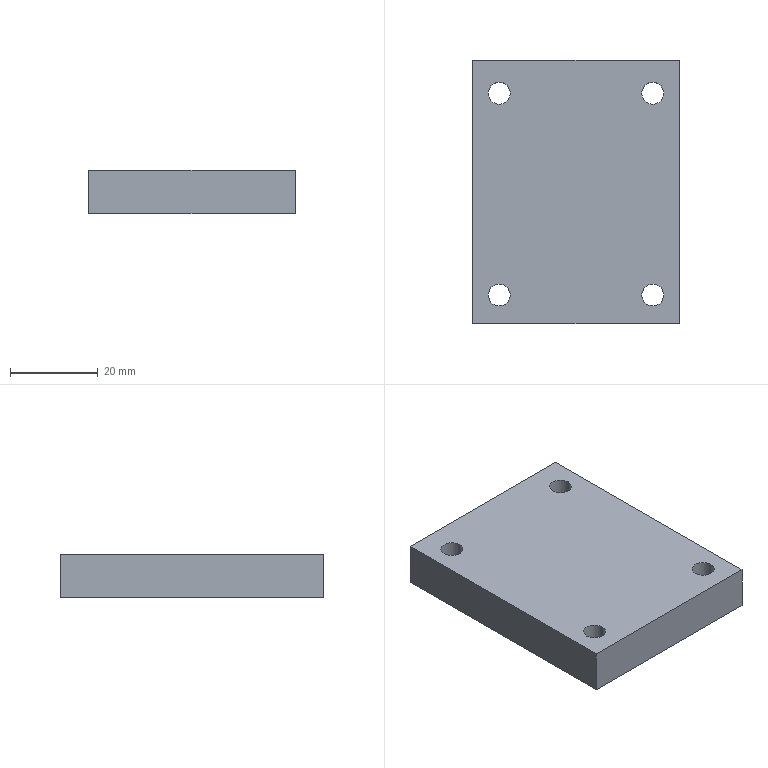Part | STEP file | X77-09109 | 1 solid | 14 faces | box 47 x 60 x 10 mm | volume 27415 mm3 | cylinder 8 | plane 6 | commonest cylinder face diameters 5 x8
STEP:
#1=CARTESIAN_POINT('',(-13.801,-204.765,0.));
#2=VERTEX_POINT('',#1);
#3=CARTESIAN_POINT('',(-18.801,-204.765,0.));
#4=VERTEX_POINT('',#3);
#5=CARTESIAN_POINT('',(-16.301,-204.765,0.));
#6=DIRECTION('',(0.,0.,-1.));
#7=DIRECTION('',(-1.,0.,0.));
#8=AXIS2_PLACEMENT_3D('',#5,#6,#7);
#9=CIRCLE('',#8,2.5);
#10=EDGE_CURVE('',#2,#4,#9,.T.);
#11=ORIENTED_EDGE('',*,*,#10,.T.);
#12=CARTESIAN_POINT('',(-18.801,-204.765,10.));
#13=VERTEX_POINT('',#12);
#14=CARTESIAN_POINT('',(-18.801,-204.765,10.));
#15=DIRECTION('',(0.,0.,1.));
#16=VECTOR('',#15,1000.);
#17=LINE('',#14,#16);
#18=EDGE_CURVE('',#4,#13,#17,.T.);
#19=ORIENTED_EDGE('',*,*,#18,.T.);
#20=CARTESIAN_POINT('',(-13.801,-204.765,10.));
#21=VERTEX_POINT('',#20);
#22=CARTESIAN_POINT('',(-16.301,-204.765,10.));
#23=DIRECTION('',(0.,0.,1.));
#24=DIRECTION('',(1.,0.,0.));
#25=AXIS2_PLACEMENT_3D('',#22,#23,#24);
#26=CIRCLE('',#25,2.5);
#27=EDGE_CURVE('',#13,#21,#26,.T.);
#28=ORIENTED_EDGE('',*,*,#27,.T.);
#29=CARTESIAN_POINT('',(-13.801,-204.765,10.));
#30=DIRECTION('',(0.,0.,1.));
#31=VECTOR('',#30,1000.);
#32=LINE('',#29,#31);
#33=EDGE_CURVE('',#2,#21,#32,.T.);
#34=ORIENTED_EDGE('',*,*,#33,.F.);
#35=EDGE_LOOP('',(#11,#19,#28,#34));
#36=FACE_OUTER_BOUND('',#35,.T.);
#37=CARTESIAN_POINT('',(-16.301,-204.765,10.));
#38=DIRECTION('',(0.,0.,1.));
#39=DIRECTION('',(1.,0.,0.));
#40=AXIS2_PLACEMENT_3D('',#37,#38,#39);
#41=CYLINDRICAL_SURFACE('',#40,2.5);
#42=ADVANCED_FACE('',(#36),#41,.F.);
#43=CARTESIAN_POINT('',(21.199,-204.765,0.));
#44=VERTEX_POINT('',#43);
#45=CARTESIAN_POINT('',(16.199,-204.765,0.));
#46=VERTEX_POINT('',#45);
#47=CARTESIAN_POINT('',(18.699,-204.765,0.));
#48=DIRECTION('',(0.,0.,-1.));
#49=DIRECTION('',(-1.,0.,0.));
#50=AXIS2_PLACEMENT_3D('',#47,#48,#49);
#51=CIRCLE('',#50,2.5);
#52=EDGE_CURVE('',#44,#46,#51,.T.);
#53=ORIENTED_EDGE('',*,*,#52,.T.);
#54=CARTESIAN_POINT('',(16.199,-204.765,10.));
#55=VERTEX_POINT('',#54);
#56=CARTESIAN_POINT('',(16.199,-204.765,10.));
#57=DIRECTION('',(0.,0.,1.));
#58=VECTOR('',#57,1000.);
#59=LINE('',#56,#58);
#60=EDGE_CURVE('',#46,#55,#59,.T.);
#61=ORIENTED_EDGE('',*,*,#60,.T.);
#62=CARTESIAN_POINT('',(21.199,-204.765,10.));
#63=VERTEX_POINT('',#62);
#64=CARTESIAN_POINT('',(18.699,-204.765,10.));
#65=DIRECTION('',(0.,0.,1.));
#66=DIRECTION('',(1.,0.,0.));
#67=AXIS2_PLACEMENT_3D('',#64,#65,#66);
#68=CIRCLE('',#67,2.5);
#69=EDGE_CURVE('',#55,#63,#68,.T.);
#70=ORIENTED_EDGE('',*,*,#69,.T.);
#71=CARTESIAN_POINT('',(21.199,-204.765,10.));
#72=DIRECTION('',(0.,0.,1.));
#73=VECTOR('',#72,1000.);
#74=LINE('',#71,#73);
#75=EDGE_CURVE('',#44,#63,#74,.T.);
#76=ORIENTED_EDGE('',*,*,#75,.F.);
#77=EDGE_LOOP('',(#53,#61,#70,#76));
#78=FACE_OUTER_BOUND('',#77,.T.);
#79=CARTESIAN_POINT('',(18.699,-204.765,10.));
#80=DIRECTION('',(0.,0.,1.));
#81=DIRECTION('',(1.,0.,0.));
#82=AXIS2_PLACEMENT_3D('',#79,#80,#81);
#83=CYLINDRICAL_SURFACE('',#82,2.5);
#84=ADVANCED_FACE('',(#78),#83,.F.);
#85=CARTESIAN_POINT('',(-13.801,-250.765,0.));
#86=VERTEX_POINT('',#85);
#87=CARTESIAN_POINT('',(-18.801,-250.765,0.));
#88=VERTEX_POINT('',#87);
#89=CARTESIAN_POINT('',(-16.301,-250.765,0.));
#90=DIRECTION('',(0.,0.,-1.));
#91=DIRECTION('',(-1.,0.,0.));
#92=AXIS2_PLACEMENT_3D('',#89,#90,#91);
#93=CIRCLE('',#92,2.5);
#94=EDGE_CURVE('',#86,#88,#93,.T.);
#95=ORIENTED_EDGE('',*,*,#94,.T.);
#96=CARTESIAN_POINT('',(-18.801,-250.765,10.));
#97=VERTEX_POINT('',#96);
#98=CARTESIAN_POINT('',(-18.801,-250.765,10.));
#99=DIRECTION('',(0.,0.,1.));
#100=VECTOR('',#99,1000.);
#101=LINE('',#98,#100);
#102=EDGE_CURVE('',#88,#97,#101,.T.);
#103=ORIENTED_EDGE('',*,*,#102,.T.);
#104=CARTESIAN_POINT('',(-13.801,-250.765,10.));
#105=VERTEX_POINT('',#104);
#106=CARTESIAN_POINT('',(-16.301,-250.765,10.));
#107=DIRECTION('',(0.,0.,1.));
#108=DIRECTION('',(1.,0.,0.));
#109=AXIS2_PLACEMENT_3D('',#106,#107,#108);
#110=CIRCLE('',#109,2.5);
#111=EDGE_CURVE('',#97,#105,#110,.T.);
#112=ORIENTED_EDGE('',*,*,#111,.T.);
#113=CARTESIAN_POINT('',(-13.801,-250.765,10.));
#114=DIRECTION('',(0.,0.,1.));
#115=VECTOR('',#114,1000.);
#116=LINE('',#113,#115);
#117=EDGE_CURVE('',#86,#105,#116,.T.);
#118=ORIENTED_EDGE('',*,*,#117,.F.);
#119=EDGE_LOOP('',(#95,#103,#112,#118));
#120=FACE_OUTER_BOUND('',#119,.T.);
#121=CARTESIAN_POINT('',(-16.301,-250.765,10.));
#122=DIRECTION('',(0.,0.,1.));
#123=DIRECTION('',(1.,0.,0.));
#124=AXIS2_PLACEMENT_3D('',#121,#122,#123);
#125=CYLINDRICAL_SURFACE('',#124,2.5);
#126=ADVANCED_FACE('',(#120),#125,.F.);
#127=CARTESIAN_POINT('',(21.199,-250.765,0.));
#128=VERTEX_POINT('',#127);
#129=CARTESIAN_POINT('',(16.199,-250.765,0.));
#130=VERTEX_POINT('',#129);
#131=CARTESIAN_POINT('',(18.699,-250.765,0.));
#132=DIRECTION('',(0.,0.,-1.));
#133=DIRECTION('',(-1.,0.,0.));
#134=AXIS2_PLACEMENT_3D('',#131,#132,#133);
#135=CIRCLE('',#134,2.5);
#136=EDGE_CURVE('',#128,#130,#135,.T.);
#137=ORIENTED_EDGE('',*,*,#136,.T.);
#138=CARTESIAN_POINT('',(16.199,-250.765,10.));
#139=VERTEX_POINT('',#138);
#140=CARTESIAN_POINT('',(16.199,-250.765,10.));
#141=DIRECTION('',(0.,0.,1.));
#142=VECTOR('',#141,1000.);
#143=LINE('',#140,#142);
#144=EDGE_CURVE('',#130,#139,#143,.T.);
#145=ORIENTED_EDGE('',*,*,#144,.T.);
#146=CARTESIAN_POINT('',(21.199,-250.765,10.));
#147=VERTEX_POINT('',#146);
#148=CARTESIAN_POINT('',(18.699,-250.765,10.));
#149=DIRECTION('',(0.,0.,1.));
#150=DIRECTION('',(1.,0.,0.));
#151=AXIS2_PLACEMENT_3D('',#148,#149,#150);
#152=CIRCLE('',#151,2.5);
#153=EDGE_CURVE('',#139,#147,#152,.T.);
#154=ORIENTED_EDGE('',*,*,#153,.T.);
#155=CARTESIAN_POINT('',(21.199,-250.765,10.));
#156=DIRECTION('',(0.,0.,1.));
#157=VECTOR('',#156,1000.);
#158=LINE('',#155,#157);
#159=EDGE_CURVE('',#128,#147,#158,.T.);
#160=ORIENTED_EDGE('',*,*,#159,.F.);
#161=EDGE_LOOP('',(#137,#145,#154,#160));
#162=FACE_OUTER_BOUND('',#161,.T.);
#163=CARTESIAN_POINT('',(18.699,-250.765,10.));
#164=DIRECTION('',(0.,0.,1.));
#165=DIRECTION('',(1.,0.,0.));
#166=AXIS2_PLACEMENT_3D('',#163,#164,#165);
#167=CYLINDRICAL_SURFACE('',#166,2.5);
#168=ADVANCED_FACE('',(#162),#167,.F.);
#169=CARTESIAN_POINT('',(24.699,-257.265,0.));
#170=VERTEX_POINT('',#169);
#171=CARTESIAN_POINT('',(24.699,-197.265,0.));
#172=VERTEX_POINT('',#171);
#173=CARTESIAN_POINT('',(24.699,-197.265,0.));
#174=DIRECTION('',(0.,1.,0.));
#175=VECTOR('',#174,1000.);
#176=LINE('',#173,#175);
#177=EDGE_CURVE('',#170,#172,#176,.T.);
#178=ORIENTED_EDGE('',*,*,#177,.T.);
#179=CARTESIAN_POINT('',(24.699,-197.265,10.));
#180=VERTEX_POINT('',#179);
#181=CARTESIAN_POINT('',(24.699,-197.265,10.));
#182=DIRECTION('',(0.,0.,-1.));
#183=VECTOR('',#182,1000.);
#184=LINE('',#181,#183);
#185=EDGE_CURVE('',#180,#172,#184,.T.);
#186=ORIENTED_EDGE('',*,*,#185,.F.);
#187=CARTESIAN_POINT('',(24.699,-257.265,10.));
#188=VERTEX_POINT('',#187);
#189=CARTESIAN_POINT('',(24.699,-197.265,10.));
#190=DIRECTION('',(0.,1.,0.));
#191=VECTOR('',#190,1000.);
#192=LINE('',#189,#191);
#193=EDGE_CURVE('',#188,#180,#192,.T.);
#194=ORIENTED_EDGE('',*,*,#193,.F.);
#195=CARTESIAN_POINT('',(24.699,-257.265,10.));
#196=DIRECTION('',(0.,0.,-1.));
#197=VECTOR('',#196,1000.);
#198=LINE('',#195,#197);
#199=EDGE_CURVE('',#188,#170,#198,.T.);
#200=ORIENTED_EDGE('',*,*,#199,.T.);
#201=EDGE_LOOP('',(#178,#186,#194,#200));
#202=FACE_OUTER_BOUND('',#201,.T.);
#203=CARTESIAN_POINT('',(24.699,-197.265,10.));
#204=DIRECTION('',(-1.,0.,0.));
#205=DIRECTION('',(0.,-1.,0.));
#206=AXIS2_PLACEMENT_3D('',#203,#204,#205);
#207=PLANE('',#206);
#208=ADVANCED_FACE('',(#202),#207,.F.);
#209=CARTESIAN_POINT('',(-22.301,-197.265,0.));
#210=VERTEX_POINT('',#209);
#211=CARTESIAN_POINT('',(24.699,-197.265,0.));
#212=DIRECTION('',(-1.,0.,0.));
#213=VECTOR('',#212,1000.);
#214=LINE('',#211,#213);
#215=EDGE_CURVE('',#172,#210,#214,.T.);
#216=ORIENTED_EDGE('',*,*,#215,.T.);
#217=CARTESIAN_POINT('',(-22.301,-197.265,10.));
#218=VERTEX_POINT('',#217);
#219=CARTESIAN_POINT('',(-22.301,-197.265,10.));
#220=DIRECTION('',(0.,0.,-1.));
#221=VECTOR('',#220,1000.);
#222=LINE('',#219,#221);
#223=EDGE_CURVE('',#218,#210,#222,.T.);
#224=ORIENTED_EDGE('',*,*,#223,.F.);
#225=CARTESIAN_POINT('',(24.699,-197.265,10.));
#226=DIRECTION('',(-1.,0.,0.));
#227=VECTOR('',#226,1000.);
#228=LINE('',#225,#227);
#229=EDGE_CURVE('',#180,#218,#228,.T.);
#230=ORIENTED_EDGE('',*,*,#229,.F.);
#231=ORIENTED_EDGE('',*,*,#185,.T.);
#232=EDGE_LOOP('',(#216,#224,#230,#231));
#233=FACE_OUTER_BOUND('',#232,.T.);
#234=CARTESIAN_POINT('',(24.699,-197.265,10.));
#235=DIRECTION('',(0.,-1.,0.));
#236=DIRECTION('',(0.,0.,-1.));
#237=AXIS2_PLACEMENT_3D('',#234,#235,#236);
#238=PLANE('',#237);
#239=ADVANCED_FACE('',(#233),#238,.F.);
#240=CARTESIAN_POINT('',(-22.301,-257.265,0.));
#241=VERTEX_POINT('',#240);
#242=CARTESIAN_POINT('',(-22.301,-197.265,0.));
#243=DIRECTION('',(0.,-1.,0.));
#244=VECTOR('',#243,1000.);
#245=LINE('',#242,#244);
#246=EDGE_CURVE('',#210,#241,#245,.T.);
#247=ORIENTED_EDGE('',*,*,#246,.T.);
#248=CARTESIAN_POINT('',(-22.301,-257.265,10.));
#249=VERTEX_POINT('',#248);
#250=CARTESIAN_POINT('',(-22.301,-257.265,10.));
#251=DIRECTION('',(0.,0.,-1.));
#252=VECTOR('',#251,1000.);
#253=LINE('',#250,#252);
#254=EDGE_CURVE('',#249,#241,#253,.T.);
#255=ORIENTED_EDGE('',*,*,#254,.F.);
#256=CARTESIAN_POINT('',(-22.301,-197.265,10.));
#257=DIRECTION('',(0.,-1.,0.));
#258=VECTOR('',#257,1000.);
#259=LINE('',#256,#258);
#260=EDGE_CURVE('',#218,#249,#259,.T.);
#261=ORIENTED_EDGE('',*,*,#260,.F.);
#262=ORIENTED_EDGE('',*,*,#223,.T.);
#263=EDGE_LOOP('',(#247,#255,#261,#262));
#264=FACE_OUTER_BOUND('',#263,.T.);
#265=CARTESIAN_POINT('',(-22.301,-197.265,10.));
#266=DIRECTION('',(1.,0.,0.));
#267=DIRECTION('',(0.,1.,0.));
#268=AXIS2_PLACEMENT_3D('',#265,#266,#267);
#269=PLANE('',#268);
#270=ADVANCED_FACE('',(#264),#269,.F.);
#271=CARTESIAN_POINT('',(24.699,-257.265,0.));
#272=DIRECTION('',(1.,0.,0.));
#273=VECTOR('',#272,1000.);
#274=LINE('',#271,#273);
#275=EDGE_CURVE('',#241,#170,#274,.T.);
#276=ORIENTED_EDGE('',*,*,#275,.T.);
#277=ORIENTED_EDGE('',*,*,#199,.F.);
#278=CARTESIAN_POINT('',(24.699,-257.265,10.));
#279=DIRECTION('',(1.,0.,0.));
#280=VECTOR('',#279,1000.);
#281=LINE('',#278,#280);
#282=EDGE_CURVE('',#249,#188,#281,.T.);
#283=ORIENTED_EDGE('',*,*,#282,.F.);
#284=ORIENTED_EDGE('',*,*,#254,.T.);
#285=EDGE_LOOP('',(#276,#277,#283,#284));
#286=FACE_OUTER_BOUND('',#285,.T.);
#287=CARTESIAN_POINT('',(24.699,-257.265,10.));
#288=DIRECTION('',(0.,1.,0.));
#289=DIRECTION('',(0.,0.,1.));
#290=AXIS2_PLACEMENT_3D('',#287,#288,#289);
#291=PLANE('',#290);
#292=ADVANCED_FACE('',(#286),#291,.F.);
#293=CARTESIAN_POINT('',(-16.301,-204.765,10.));
#294=DIRECTION('',(0.,0.,1.));
#295=DIRECTION('',(1.,0.,0.));
#296=AXIS2_PLACEMENT_3D('',#293,#294,#295);
#297=CIRCLE('',#296,2.5);
#298=EDGE_CURVE('',#21,#13,#297,.T.);
#299=ORIENTED_EDGE('',*,*,#298,.F.);
#300=ORIENTED_EDGE('',*,*,#27,.F.);
#301=EDGE_LOOP('',(#299,#300));
#302=FACE_BOUND('',#301,.T.);
#303=CARTESIAN_POINT('',(18.699,-204.765,10.));
#304=DIRECTION('',(0.,0.,1.));
#305=DIRECTION('',(1.,0.,0.));
#306=AXIS2_PLACEMENT_3D('',#303,#304,#305);
#307=CIRCLE('',#306,2.5);
#308=EDGE_CURVE('',#63,#55,#307,.T.);
#309=ORIENTED_EDGE('',*,*,#308,.F.);
#310=ORIENTED_EDGE('',*,*,#69,.F.);
#311=EDGE_LOOP('',(#309,#310));
#312=FACE_BOUND('',#311,.T.);
#313=CARTESIAN_POINT('',(-16.301,-250.765,10.));
#314=DIRECTION('',(0.,0.,1.));
#315=DIRECTION('',(1.,0.,0.));
#316=AXIS2_PLACEMENT_3D('',#313,#314,#315);
#317=CIRCLE('',#316,2.5);
#318=EDGE_CURVE('',#105,#97,#317,.T.);
#319=ORIENTED_EDGE('',*,*,#318,.F.);
#320=ORIENTED_EDGE('',*,*,#111,.F.);
#321=EDGE_LOOP('',(#319,#320));
#322=FACE_BOUND('',#321,.T.);
#323=CARTESIAN_POINT('',(18.699,-250.765,10.));
#324=DIRECTION('',(0.,0.,1.));
#325=DIRECTION('',(1.,0.,0.));
#326=AXIS2_PLACEMENT_3D('',#323,#324,#325);
#327=CIRCLE('',#326,2.5);
#328=EDGE_CURVE('',#147,#139,#327,.T.);
#329=ORIENTED_EDGE('',*,*,#328,.F.);
#330=ORIENTED_EDGE('',*,*,#153,.F.);
#331=EDGE_LOOP('',(#329,#330));
#332=FACE_BOUND('',#331,.T.);
#333=ORIENTED_EDGE('',*,*,#193,.T.);
#334=ORIENTED_EDGE('',*,*,#229,.T.);
#335=ORIENTED_EDGE('',*,*,#260,.T.);
#336=ORIENTED_EDGE('',*,*,#282,.T.);
#337=EDGE_LOOP('',(#333,#334,#335,#336));
#338=FACE_OUTER_BOUND('',#337,.T.);
#339=CARTESIAN_POINT('',(24.699,-257.265,10.));
#340=DIRECTION('',(0.,0.,-1.));
#341=DIRECTION('',(-1.,0.,0.));
#342=AXIS2_PLACEMENT_3D('',#339,#340,#341);
#343=PLANE('',#342);
#344=ADVANCED_FACE('',(#302,#312,#322,#332,#338),#343,.F.);
#345=ORIENTED_EDGE('',*,*,#10,.F.);
#346=CARTESIAN_POINT('',(-16.301,-204.765,0.));
#347=DIRECTION('',(0.,0.,-1.));
#348=DIRECTION('',(-1.,0.,0.));
#349=AXIS2_PLACEMENT_3D('',#346,#347,#348);
#350=CIRCLE('',#349,2.5);
#351=EDGE_CURVE('',#4,#2,#350,.T.);
#352=ORIENTED_EDGE('',*,*,#351,.F.);
#353=EDGE_LOOP('',(#345,#352));
#354=FACE_BOUND('',#353,.T.);
#355=ORIENTED_EDGE('',*,*,#52,.F.);
#356=CARTESIAN_POINT('',(18.699,-204.765,0.));
#357=DIRECTION('',(0.,0.,-1.));
#358=DIRECTION('',(-1.,0.,0.));
#359=AXIS2_PLACEMENT_3D('',#356,#357,#358);
#360=CIRCLE('',#359,2.5);
#361=EDGE_CURVE('',#46,#44,#360,.T.);
#362=ORIENTED_EDGE('',*,*,#361,.F.);
#363=EDGE_LOOP('',(#355,#362));
#364=FACE_BOUND('',#363,.T.);
#365=ORIENTED_EDGE('',*,*,#94,.F.);
#366=CARTESIAN_POINT('',(-16.301,-250.765,0.));
#367=DIRECTION('',(0.,0.,-1.));
#368=DIRECTION('',(-1.,0.,0.));
#369=AXIS2_PLACEMENT_3D('',#366,#367,#368);
#370=CIRCLE('',#369,2.5);
#371=EDGE_CURVE('',#88,#86,#370,.T.);
#372=ORIENTED_EDGE('',*,*,#371,.F.);
#373=EDGE_LOOP('',(#365,#372));
#374=FACE_BOUND('',#373,.T.);
#375=ORIENTED_EDGE('',*,*,#136,.F.);
#376=CARTESIAN_POINT('',(18.699,-250.765,0.));
#377=DIRECTION('',(0.,0.,-1.));
#378=DIRECTION('',(-1.,0.,0.));
#379=AXIS2_PLACEMENT_3D('',#376,#377,#378);
#380=CIRCLE('',#379,2.5);
#381=EDGE_CURVE('',#130,#128,#380,.T.);
#382=ORIENTED_EDGE('',*,*,#381,.F.);
#383=EDGE_LOOP('',(#375,#382));
#384=FACE_BOUND('',#383,.T.);
#385=ORIENTED_EDGE('',*,*,#177,.F.);
#386=ORIENTED_EDGE('',*,*,#275,.F.);
#387=ORIENTED_EDGE('',*,*,#246,.F.);
#388=ORIENTED_EDGE('',*,*,#215,.F.);
#389=EDGE_LOOP('',(#385,#386,#387,#388));
#390=FACE_OUTER_BOUND('',#389,.T.);
#391=CARTESIAN_POINT('',(24.699,-257.265,0.));
#392=DIRECTION('',(0.,0.,-1.));
#393=DIRECTION('',(-1.,0.,0.));
#394=AXIS2_PLACEMENT_3D('',#391,#392,#393);
#395=PLANE('',#394);
#396=ADVANCED_FACE('',(#354,#364,#374,#384,#390),#395,.T.);
#397=ORIENTED_EDGE('',*,*,#144,.F.);
#398=ORIENTED_EDGE('',*,*,#381,.T.);
#399=ORIENTED_EDGE('',*,*,#159,.T.);
#400=ORIENTED_EDGE('',*,*,#328,.T.);
#401=EDGE_LOOP('',(#397,#398,#399,#400));
#402=FACE_OUTER_BOUND('',#401,.T.);
#403=CARTESIAN_POINT('',(18.699,-250.765,10.));
#404=DIRECTION('',(0.,0.,1.));
#405=DIRECTION('',(1.,0.,0.));
#406=AXIS2_PLACEMENT_3D('',#403,#404,#405);
#407=CYLINDRICAL_SURFACE('',#406,2.5);
#408=ADVANCED_FACE('',(#402),#407,.F.);
#409=ORIENTED_EDGE('',*,*,#102,.F.);
#410=ORIENTED_EDGE('',*,*,#371,.T.);
#411=ORIENTED_EDGE('',*,*,#117,.T.);
#412=ORIENTED_EDGE('',*,*,#318,.T.);
#413=EDGE_LOOP('',(#409,#410,#411,#412));
#414=FACE_OUTER_BOUND('',#413,.T.);
#415=CARTESIAN_POINT('',(-16.301,-250.765,10.));
#416=DIRECTION('',(0.,0.,1.));
#417=DIRECTION('',(1.,0.,0.));
#418=AXIS2_PLACEMENT_3D('',#415,#416,#417);
#419=CYLINDRICAL_SURFACE('',#418,2.5);
#420=ADVANCED_FACE('',(#414),#419,.F.);
#421=ORIENTED_EDGE('',*,*,#60,.F.);
#422=ORIENTED_EDGE('',*,*,#361,.T.);
#423=ORIENTED_EDGE('',*,*,#75,.T.);
#424=ORIENTED_EDGE('',*,*,#308,.T.);
#425=EDGE_LOOP('',(#421,#422,#423,#424));
#426=FACE_OUTER_BOUND('',#425,.T.);
#427=CARTESIAN_POINT('',(18.699,-204.765,10.));
#428=DIRECTION('',(0.,0.,1.));
#429=DIRECTION('',(1.,0.,0.));
#430=AXIS2_PLACEMENT_3D('',#427,#428,#429);
#431=CYLINDRICAL_SURFACE('',#430,2.5);
#432=ADVANCED_FACE('',(#426),#431,.F.);
#433=ORIENTED_EDGE('',*,*,#18,.F.);
#434=ORIENTED_EDGE('',*,*,#351,.T.);
#435=ORIENTED_EDGE('',*,*,#33,.T.);
#436=ORIENTED_EDGE('',*,*,#298,.T.);
#437=EDGE_LOOP('',(#433,#434,#435,#436));
#438=FACE_OUTER_BOUND('',#437,.T.);
#439=CARTESIAN_POINT('',(-16.301,-204.765,10.));
#440=DIRECTION('',(0.,0.,1.));
#441=DIRECTION('',(1.,0.,0.));
#442=AXIS2_PLACEMENT_3D('',#439,#440,#441);
#443=CYLINDRICAL_SURFACE('',#442,2.5);
#444=ADVANCED_FACE('',(#438),#443,.F.);
#445=CLOSED_SHELL('',(#42,#84,#126,#168,#208,#239,#270,#292,#344,#396,#408,#420,#432,#444));
#446=MANIFOLD_SOLID_BREP('',#445);
#447=CARTESIAN_POINT('',(0.,0.,0.));
#448=DIRECTION('',(0.,0.,1.));
#449=DIRECTION('',(1.,0.,0.));
#450=AXIS2_PLACEMENT_3D('',#447,#448,#449);
#451=(LENGTH_UNIT()NAMED_UNIT(*)SI_UNIT(.MILLI.,.METRE.));
#452=UNCERTAINTY_MEASURE_WITH_UNIT(LENGTH_MEASURE(0.00001),#451,'','');
#453=(NAMED_UNIT(*)PLANE_ANGLE_UNIT()SI_UNIT($,.RADIAN.));
#454=(NAMED_UNIT(*)SI_UNIT($,.STERADIAN.)SOLID_ANGLE_UNIT());
#455=(GEOMETRIC_REPRESENTATION_CONTEXT(3)GLOBAL_UNCERTAINTY_ASSIGNED_CONTEXT((#452))GLOBAL_UNIT_ASSIGNED_CONTEXT((#451,#453,#454))REPRESENTATION_CONTEXT('',''));
#456=ADVANCED_BREP_SHAPE_REPRESENTATION('',(#446,#450),#455);